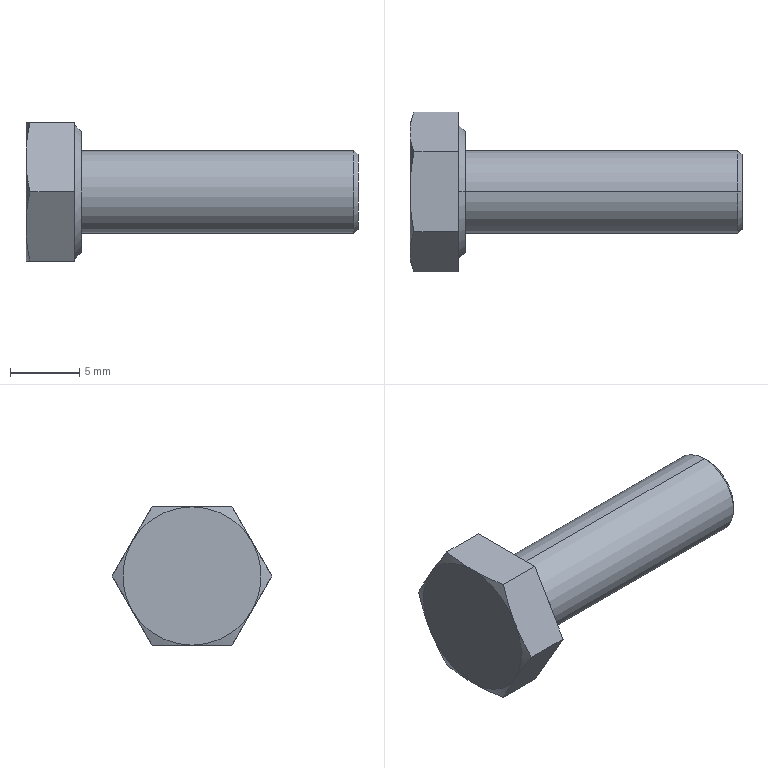Part | STEP file | hex head bolts-full thread grade c gb_GB_FASTENER_BOLT_HHBFTC M6X20-S | 1 solid | 22 faces | box 24 x 11.547 x 10 mm | volume 900.64 mm3 | cone 10 | plane 10 | cylinder 2 | commonest cylinder face diameters 6 x2
STEP:
#1=CARTESIAN_POINT('',(23.7,0.,3.));
#2=VERTEX_POINT('',#1);
#3=CARTESIAN_POINT('',(23.7,0.,-3.));
#4=VERTEX_POINT('',#3);
#5=CARTESIAN_POINT('',(23.7,0.,0.));
#6=DIRECTION('',(-1.,0.,0.));
#7=DIRECTION('',(0.,0.,1.));
#8=AXIS2_PLACEMENT_3D('',#5,#6,#7);
#9=CIRCLE('',#8,3.);
#10=EDGE_CURVE('',#2,#4,#9,.T.);
#11=ORIENTED_EDGE('',*,*,#10,.T.);
#12=CARTESIAN_POINT('',(4.,0.,-3.));
#13=VERTEX_POINT('',#12);
#14=CARTESIAN_POINT('',(24.,0.,-3.));
#15=DIRECTION('',(-1.,0.,0.));
#16=VECTOR('',#15,1000.);
#17=LINE('',#14,#16);
#18=EDGE_CURVE('',#4,#13,#17,.T.);
#19=ORIENTED_EDGE('',*,*,#18,.T.);
#20=CARTESIAN_POINT('',(4.,0.,3.));
#21=VERTEX_POINT('',#20);
#22=CARTESIAN_POINT('',(4.,0.,0.));
#23=DIRECTION('',(1.,0.,0.));
#24=DIRECTION('',(0.,0.,1.));
#25=AXIS2_PLACEMENT_3D('',#22,#23,#24);
#26=CIRCLE('',#25,3.);
#27=EDGE_CURVE('',#13,#21,#26,.T.);
#28=ORIENTED_EDGE('',*,*,#27,.T.);
#29=CARTESIAN_POINT('',(24.,0.,3.));
#30=DIRECTION('',(-1.,0.,0.));
#31=VECTOR('',#30,1000.);
#32=LINE('',#29,#31);
#33=EDGE_CURVE('',#2,#21,#32,.T.);
#34=ORIENTED_EDGE('',*,*,#33,.F.);
#35=EDGE_LOOP('',(#11,#19,#28,#34));
#36=FACE_OUTER_BOUND('',#35,.T.);
#37=CARTESIAN_POINT('',(24.,0.,0.));
#38=DIRECTION('',(-1.,0.,0.));
#39=DIRECTION('',(0.,0.,1.));
#40=AXIS2_PLACEMENT_3D('',#37,#38,#39);
#41=CYLINDRICAL_SURFACE('',#40,3.);
#42=ADVANCED_FACE('',(#36),#41,.T.);
#43=CARTESIAN_POINT('',(24.,0.,2.7));
#44=VERTEX_POINT('',#43);
#45=CARTESIAN_POINT('',(24.,0.,-2.7));
#46=VERTEX_POINT('',#45);
#47=CARTESIAN_POINT('',(24.,0.,0.));
#48=DIRECTION('',(-1.,0.,0.));
#49=DIRECTION('',(0.,0.,1.));
#50=AXIS2_PLACEMENT_3D('',#47,#48,#49);
#51=CIRCLE('',#50,2.7);
#52=EDGE_CURVE('',#44,#46,#51,.T.);
#53=ORIENTED_EDGE('',*,*,#52,.T.);
#54=CARTESIAN_POINT('',(23.7,0.,-3.));
#55=DIRECTION('',(-0.7071,0.,-0.7071));
#56=VECTOR('',#55,1000.);
#57=LINE('',#54,#56);
#58=EDGE_CURVE('',#46,#4,#57,.T.);
#59=ORIENTED_EDGE('',*,*,#58,.T.);
#60=ORIENTED_EDGE('',*,*,#10,.F.);
#61=CARTESIAN_POINT('',(23.7,0.,3.));
#62=DIRECTION('',(-0.7071,0.,0.7071));
#63=VECTOR('',#62,1000.);
#64=LINE('',#61,#63);
#65=EDGE_CURVE('',#44,#2,#64,.T.);
#66=ORIENTED_EDGE('',*,*,#65,.F.);
#67=EDGE_LOOP('',(#53,#59,#60,#66));
#68=FACE_OUTER_BOUND('',#67,.T.);
#69=CARTESIAN_POINT('',(23.7,0.,0.));
#70=DIRECTION('',(-1.,0.,0.));
#71=DIRECTION('',(0.,0.,1.));
#72=AXIS2_PLACEMENT_3D('',#69,#70,#71);
#73=CONICAL_SURFACE('',#72,3.,0.7854);
#74=ADVANCED_FACE('',(#68),#73,.T.);
#75=CARTESIAN_POINT('',(4.,0.,4.37));
#76=VERTEX_POINT('',#75);
#77=CARTESIAN_POINT('',(4.,0.,-4.37));
#78=VERTEX_POINT('',#77);
#79=CARTESIAN_POINT('',(4.,0.,0.));
#80=DIRECTION('',(-1.,0.,0.));
#81=DIRECTION('',(0.,0.,1.));
#82=AXIS2_PLACEMENT_3D('',#79,#80,#81);
#83=CIRCLE('',#82,4.37);
#84=EDGE_CURVE('',#76,#78,#83,.T.);
#85=ORIENTED_EDGE('',*,*,#84,.T.);
#86=CARTESIAN_POINT('',(3.5,0.,-4.87));
#87=VERTEX_POINT('',#86);
#88=CARTESIAN_POINT('',(3.5,0.,-4.87));
#89=DIRECTION('',(-0.7071,0.,-0.7071));
#90=VECTOR('',#89,1000.);
#91=LINE('',#88,#90);
#92=EDGE_CURVE('',#78,#87,#91,.T.);
#93=ORIENTED_EDGE('',*,*,#92,.T.);
#94=CARTESIAN_POINT('',(3.5,0.,4.87));
#95=VERTEX_POINT('',#94);
#96=CARTESIAN_POINT('',(3.5,0.,0.));
#97=DIRECTION('',(1.,0.,0.));
#98=DIRECTION('',(0.,0.,1.));
#99=AXIS2_PLACEMENT_3D('',#96,#97,#98);
#100=CIRCLE('',#99,4.87);
#101=EDGE_CURVE('',#87,#95,#100,.T.);
#102=ORIENTED_EDGE('',*,*,#101,.T.);
#103=CARTESIAN_POINT('',(3.5,0.,4.87));
#104=DIRECTION('',(-0.7071,0.,0.7071));
#105=VECTOR('',#104,1000.);
#106=LINE('',#103,#105);
#107=EDGE_CURVE('',#76,#95,#106,.T.);
#108=ORIENTED_EDGE('',*,*,#107,.F.);
#109=EDGE_LOOP('',(#85,#93,#102,#108));
#110=FACE_OUTER_BOUND('',#109,.T.);
#111=CARTESIAN_POINT('',(3.5,0.,0.));
#112=DIRECTION('',(-1.,0.,0.));
#113=DIRECTION('',(0.,0.,1.));
#114=AXIS2_PLACEMENT_3D('',#111,#112,#113);
#115=CONICAL_SURFACE('',#114,4.87,0.7854);
#116=ADVANCED_FACE('',(#110),#115,.T.);
#117=ORIENTED_EDGE('',*,*,#18,.F.);
#118=CARTESIAN_POINT('',(23.7,0.,0.));
#119=DIRECTION('',(-1.,0.,0.));
#120=DIRECTION('',(0.,0.,1.));
#121=AXIS2_PLACEMENT_3D('',#118,#119,#120);
#122=CIRCLE('',#121,3.);
#123=EDGE_CURVE('',#4,#2,#122,.T.);
#124=ORIENTED_EDGE('',*,*,#123,.T.);
#125=ORIENTED_EDGE('',*,*,#33,.T.);
#126=CARTESIAN_POINT('',(4.,0.,0.));
#127=DIRECTION('',(1.,0.,0.));
#128=DIRECTION('',(0.,0.,1.));
#129=AXIS2_PLACEMENT_3D('',#126,#127,#128);
#130=CIRCLE('',#129,3.);
#131=EDGE_CURVE('',#21,#13,#130,.T.);
#132=ORIENTED_EDGE('',*,*,#131,.T.);
#133=EDGE_LOOP('',(#117,#124,#125,#132));
#134=FACE_OUTER_BOUND('',#133,.T.);
#135=CARTESIAN_POINT('',(24.,0.,0.));
#136=DIRECTION('',(-1.,0.,0.));
#137=DIRECTION('',(0.,0.,1.));
#138=AXIS2_PLACEMENT_3D('',#135,#136,#137);
#139=CYLINDRICAL_SURFACE('',#138,3.);
#140=ADVANCED_FACE('',(#134),#139,.T.);
#141=ORIENTED_EDGE('',*,*,#131,.F.);
#142=ORIENTED_EDGE('',*,*,#27,.F.);
#143=EDGE_LOOP('',(#141,#142));
#144=FACE_BOUND('',#143,.T.);
#145=ORIENTED_EDGE('',*,*,#84,.F.);
#146=CARTESIAN_POINT('',(4.,0.,0.));
#147=DIRECTION('',(-1.,0.,0.));
#148=DIRECTION('',(0.,0.,1.));
#149=AXIS2_PLACEMENT_3D('',#146,#147,#148);
#150=CIRCLE('',#149,4.37);
#151=EDGE_CURVE('',#78,#76,#150,.T.);
#152=ORIENTED_EDGE('',*,*,#151,.F.);
#153=EDGE_LOOP('',(#145,#152));
#154=FACE_OUTER_BOUND('',#153,.T.);
#155=CARTESIAN_POINT('',(4.,0.,10.));
#156=DIRECTION('',(-1.,0.,0.));
#157=DIRECTION('',(0.,0.,1.));
#158=AXIS2_PLACEMENT_3D('',#155,#156,#157);
#159=PLANE('',#158);
#160=ADVANCED_FACE('',(#144,#154),#159,.F.);
#161=ORIENTED_EDGE('',*,*,#58,.F.);
#162=CARTESIAN_POINT('',(24.,0.,0.));
#163=DIRECTION('',(-1.,0.,0.));
#164=DIRECTION('',(0.,0.,1.));
#165=AXIS2_PLACEMENT_3D('',#162,#163,#164);
#166=CIRCLE('',#165,2.7);
#167=EDGE_CURVE('',#46,#44,#166,.T.);
#168=ORIENTED_EDGE('',*,*,#167,.T.);
#169=ORIENTED_EDGE('',*,*,#65,.T.);
#170=ORIENTED_EDGE('',*,*,#123,.F.);
#171=EDGE_LOOP('',(#161,#168,#169,#170));
#172=FACE_OUTER_BOUND('',#171,.T.);
#173=CARTESIAN_POINT('',(23.7,0.,0.));
#174=DIRECTION('',(-1.,0.,0.));
#175=DIRECTION('',(0.,0.,1.));
#176=AXIS2_PLACEMENT_3D('',#173,#174,#175);
#177=CONICAL_SURFACE('',#176,3.,0.7854);
#178=ADVANCED_FACE('',(#172),#177,.T.);
#179=ORIENTED_EDGE('',*,*,#92,.F.);
#180=ORIENTED_EDGE('',*,*,#151,.T.);
#181=ORIENTED_EDGE('',*,*,#107,.T.);
#182=CARTESIAN_POINT('',(3.5,0.,0.));
#183=DIRECTION('',(1.,0.,0.));
#184=DIRECTION('',(0.,0.,1.));
#185=AXIS2_PLACEMENT_3D('',#182,#183,#184);
#186=CIRCLE('',#185,4.87);
#187=EDGE_CURVE('',#95,#87,#186,.T.);
#188=ORIENTED_EDGE('',*,*,#187,.T.);
#189=EDGE_LOOP('',(#179,#180,#181,#188));
#190=FACE_OUTER_BOUND('',#189,.T.);
#191=CARTESIAN_POINT('',(3.5,0.,0.));
#192=DIRECTION('',(-1.,0.,0.));
#193=DIRECTION('',(0.,0.,1.));
#194=AXIS2_PLACEMENT_3D('',#191,#192,#193);
#195=CONICAL_SURFACE('',#194,4.87,0.7854);
#196=ADVANCED_FACE('',(#190),#195,.T.);
#197=ORIENTED_EDGE('',*,*,#52,.F.);
#198=ORIENTED_EDGE('',*,*,#167,.F.);
#199=EDGE_LOOP('',(#197,#198));
#200=FACE_OUTER_BOUND('',#199,.T.);
#201=CARTESIAN_POINT('',(24.,0.,0.));
#202=DIRECTION('',(1.,0.,0.));
#203=DIRECTION('',(0.,0.,-1.));
#204=AXIS2_PLACEMENT_3D('',#201,#202,#203);
#205=PLANE('',#204);
#206=ADVANCED_FACE('',(#200),#205,.T.);
#207=CARTESIAN_POINT('',(3.5,5.774,0.));
#208=VERTEX_POINT('',#207);
#209=CARTESIAN_POINT('',(3.5,2.887,5.));
#210=VERTEX_POINT('',#209);
#211=CARTESIAN_POINT('',(3.5,5.774,0.));
#212=DIRECTION('',(0.,-0.5,0.866));
#213=VECTOR('',#212,1000.);
#214=LINE('',#211,#213);
#215=EDGE_CURVE('',#208,#210,#214,.T.);
#216=ORIENTED_EDGE('',*,*,#215,.T.);
#217=CARTESIAN_POINT('',(3.5,-2.887,5.));
#218=VERTEX_POINT('',#217);
#219=CARTESIAN_POINT('',(3.5,4.87,5.));
#220=DIRECTION('',(0.,-1.,0.));
#221=VECTOR('',#220,1000.);
#222=LINE('',#219,#221);
#223=EDGE_CURVE('',#210,#218,#222,.T.);
#224=ORIENTED_EDGE('',*,*,#223,.T.);
#225=CARTESIAN_POINT('',(3.5,-5.774,0.));
#226=VERTEX_POINT('',#225);
#227=CARTESIAN_POINT('',(3.5,-2.887,5.));
#228=DIRECTION('',(0.,-0.5,-0.866));
#229=VECTOR('',#228,1000.);
#230=LINE('',#227,#229);
#231=EDGE_CURVE('',#218,#226,#230,.T.);
#232=ORIENTED_EDGE('',*,*,#231,.T.);
#233=CARTESIAN_POINT('',(3.5,-2.887,-5.));
#234=VERTEX_POINT('',#233);
#235=CARTESIAN_POINT('',(3.5,-5.774,0.));
#236=DIRECTION('',(0.,0.5,-0.866));
#237=VECTOR('',#236,1000.);
#238=LINE('',#235,#237);
#239=EDGE_CURVE('',#226,#234,#238,.T.);
#240=ORIENTED_EDGE('',*,*,#239,.T.);
#241=CARTESIAN_POINT('',(3.5,2.887,-5.));
#242=VERTEX_POINT('',#241);
#243=CARTESIAN_POINT('',(3.5,4.87,-5.));
#244=DIRECTION('',(0.,1.,0.));
#245=VECTOR('',#244,1000.);
#246=LINE('',#243,#245);
#247=EDGE_CURVE('',#234,#242,#246,.T.);
#248=ORIENTED_EDGE('',*,*,#247,.T.);
#249=CARTESIAN_POINT('',(3.5,2.887,-5.));
#250=DIRECTION('',(0.,0.5,0.866));
#251=VECTOR('',#250,1000.);
#252=LINE('',#249,#251);
#253=EDGE_CURVE('',#242,#208,#252,.T.);
#254=ORIENTED_EDGE('',*,*,#253,.T.);
#255=EDGE_LOOP('',(#216,#224,#232,#240,#248,#254));
#256=FACE_OUTER_BOUND('',#255,.T.);
#257=ORIENTED_EDGE('',*,*,#187,.F.);
#258=ORIENTED_EDGE('',*,*,#101,.F.);
#259=EDGE_LOOP('',(#257,#258));
#260=FACE_BOUND('',#259,.T.);
#261=CARTESIAN_POINT('',(3.5,4.87,0.));
#262=DIRECTION('',(1.,0.,0.));
#263=DIRECTION('',(0.,0.,-1.));
#264=AXIS2_PLACEMENT_3D('',#261,#262,#263);
#265=PLANE('',#264);
#266=ADVANCED_FACE('',(#256,#260),#265,.T.);
#267=CARTESIAN_POINT('',(0.2815,-2.887,5.));
#268=VERTEX_POINT('',#267);
#269=CARTESIAN_POINT('',(4.,-2.887,5.));
#270=DIRECTION('',(-1.,0.,0.));
#271=VECTOR('',#270,1000.);
#272=LINE('',#269,#271);
#273=EDGE_CURVE('',#218,#268,#272,.T.);
#274=ORIENTED_EDGE('',*,*,#273,.F.);
#275=ORIENTED_EDGE('',*,*,#223,.F.);
#276=CARTESIAN_POINT('',(0.2815,2.887,5.));
#277=VERTEX_POINT('',#276);
#278=CARTESIAN_POINT('',(4.,2.887,5.));
#279=DIRECTION('',(1.,0.,0.));
#280=VECTOR('',#279,1000.);
#281=LINE('',#278,#280);
#282=EDGE_CURVE('',#277,#210,#281,.T.);
#283=ORIENTED_EDGE('',*,*,#282,.F.);
#284=CARTESIAN_POINT('',(0.,0.,5.));
#285=VERTEX_POINT('',#284);
#286=CARTESIAN_POINT('',(0.,0.,5.));
#287=CARTESIAN_POINT('',(0.,0.9714,5.));
#288=CARTESIAN_POINT('',(0.1078,1.932,5.));
#289=CARTESIAN_POINT('',(0.2815,2.887,5.));
#290=B_SPLINE_CURVE_WITH_KNOTS('',3,(#286,#287,#288,#289),.UNSPECIFIED.,.F.,.F.,(4,4),(0.,0.0029),.UNSPECIFIED.);
#291=EDGE_CURVE('',#285,#277,#290,.T.);
#292=ORIENTED_EDGE('',*,*,#291,.F.);
#293=CARTESIAN_POINT('',(0.2815,-2.887,5.));
#294=CARTESIAN_POINT('',(0.1078,-1.932,5.));
#295=CARTESIAN_POINT('',(0.,-0.9714,5.));
#296=CARTESIAN_POINT('',(0.,0.,5.));
#297=B_SPLINE_CURVE_WITH_KNOTS('',3,(#293,#294,#295,#296),.UNSPECIFIED.,.F.,.F.,(4,4),(0.,0.0029),.UNSPECIFIED.);
#298=EDGE_CURVE('',#268,#285,#297,.T.);
#299=ORIENTED_EDGE('',*,*,#298,.F.);
#300=EDGE_LOOP('',(#274,#275,#283,#292,#299));
#301=FACE_OUTER_BOUND('',#300,.T.);
#302=CARTESIAN_POINT('',(4.,2.887,5.));
#303=DIRECTION('',(0.,0.,-1.));
#304=DIRECTION('',(0.,1.,0.));
#305=AXIS2_PLACEMENT_3D('',#302,#303,#304);
#306=PLANE('',#305);
#307=ADVANCED_FACE('',(#301),#306,.F.);
#308=ORIENTED_EDGE('',*,*,#282,.T.);
#309=ORIENTED_EDGE('',*,*,#215,.F.);
#310=CARTESIAN_POINT('',(0.2815,5.774,0.));
#311=VERTEX_POINT('',#310);
#312=CARTESIAN_POINT('',(4.,5.774,0.));
#313=DIRECTION('',(1.,0.,0.));
#314=VECTOR('',#313,1000.);
#315=LINE('',#312,#314);
#316=EDGE_CURVE('',#311,#208,#315,.T.);
#317=ORIENTED_EDGE('',*,*,#316,.F.);
#318=CARTESIAN_POINT('',(0.,4.33,2.5));
#319=VERTEX_POINT('',#318);
#320=CARTESIAN_POINT('',(0.,4.33,2.5));
#321=CARTESIAN_POINT('',(0.,4.816,1.659));
#322=CARTESIAN_POINT('',(0.1078,5.296,0.8266));
#323=CARTESIAN_POINT('',(0.2815,5.774,0.));
#324=B_SPLINE_CURVE_WITH_KNOTS('',3,(#320,#321,#322,#323),.UNSPECIFIED.,.F.,.F.,(4,4),(0.,0.0029),.UNSPECIFIED.);
#325=EDGE_CURVE('',#319,#311,#324,.T.);
#326=ORIENTED_EDGE('',*,*,#325,.F.);
#327=CARTESIAN_POINT('',(0.2815,2.887,5.));
#328=CARTESIAN_POINT('',(0.1078,3.364,4.173));
#329=CARTESIAN_POINT('',(0.,3.844,3.341));
#330=CARTESIAN_POINT('',(0.,4.33,2.5));
#331=B_SPLINE_CURVE_WITH_KNOTS('',3,(#327,#328,#329,#330),.UNSPECIFIED.,.F.,.F.,(4,4),(0.,0.0029),.UNSPECIFIED.);
#332=EDGE_CURVE('',#277,#319,#331,.T.);
#333=ORIENTED_EDGE('',*,*,#332,.F.);
#334=EDGE_LOOP('',(#308,#309,#317,#326,#333));
#335=FACE_OUTER_BOUND('',#334,.T.);
#336=CARTESIAN_POINT('',(4.,5.774,0.));
#337=DIRECTION('',(0.,-0.866,-0.5));
#338=DIRECTION('',(0.,0.5,-0.866));
#339=AXIS2_PLACEMENT_3D('',#336,#337,#338);
#340=PLANE('',#339);
#341=ADVANCED_FACE('',(#335),#340,.F.);
#342=ORIENTED_EDGE('',*,*,#316,.T.);
#343=ORIENTED_EDGE('',*,*,#253,.F.);
#344=CARTESIAN_POINT('',(0.2815,2.887,-5.));
#345=VERTEX_POINT('',#344);
#346=CARTESIAN_POINT('',(4.,2.887,-5.));
#347=DIRECTION('',(1.,0.,0.));
#348=VECTOR('',#347,1000.);
#349=LINE('',#346,#348);
#350=EDGE_CURVE('',#345,#242,#349,.T.);
#351=ORIENTED_EDGE('',*,*,#350,.F.);
#352=CARTESIAN_POINT('',(0.,4.33,-2.5));
#353=VERTEX_POINT('',#352);
#354=CARTESIAN_POINT('',(0.,4.33,-2.5));
#355=CARTESIAN_POINT('',(0.,3.844,-3.341));
#356=CARTESIAN_POINT('',(0.1078,3.364,-4.173));
#357=CARTESIAN_POINT('',(0.2815,2.887,-5.));
#358=B_SPLINE_CURVE_WITH_KNOTS('',3,(#354,#355,#356,#357),.UNSPECIFIED.,.F.,.F.,(4,4),(0.,0.0029),.UNSPECIFIED.);
#359=EDGE_CURVE('',#353,#345,#358,.T.);
#360=ORIENTED_EDGE('',*,*,#359,.F.);
#361=CARTESIAN_POINT('',(0.2815,5.774,0.));
#362=CARTESIAN_POINT('',(0.1078,5.296,-0.8266));
#363=CARTESIAN_POINT('',(0.,4.816,-1.659));
#364=CARTESIAN_POINT('',(0.,4.33,-2.5));
#365=B_SPLINE_CURVE_WITH_KNOTS('',3,(#361,#362,#363,#364),.UNSPECIFIED.,.F.,.F.,(4,4),(0.,0.0029),.UNSPECIFIED.);
#366=EDGE_CURVE('',#311,#353,#365,.T.);
#367=ORIENTED_EDGE('',*,*,#366,.F.);
#368=EDGE_LOOP('',(#342,#343,#351,#360,#367));
#369=FACE_OUTER_BOUND('',#368,.T.);
#370=CARTESIAN_POINT('',(4.,2.887,-5.));
#371=DIRECTION('',(0.,-0.866,0.5));
#372=DIRECTION('',(0.,-0.5,-0.866));
#373=AXIS2_PLACEMENT_3D('',#370,#371,#372);
#374=PLANE('',#373);
#375=ADVANCED_FACE('',(#369),#374,.F.);
#376=ORIENTED_EDGE('',*,*,#350,.T.);
#377=ORIENTED_EDGE('',*,*,#247,.F.);
#378=CARTESIAN_POINT('',(0.2815,-2.887,-5.));
#379=VERTEX_POINT('',#378);
#380=CARTESIAN_POINT('',(4.,-2.887,-5.));
#381=DIRECTION('',(1.,0.,0.));
#382=VECTOR('',#381,1000.);
#383=LINE('',#380,#382);
#384=EDGE_CURVE('',#379,#234,#383,.T.);
#385=ORIENTED_EDGE('',*,*,#384,.F.);
#386=CARTESIAN_POINT('',(0.,0.,-5.));
#387=VERTEX_POINT('',#386);
#388=CARTESIAN_POINT('',(0.,0.,-5.));
#389=CARTESIAN_POINT('',(0.,-0.9714,-5.));
#390=CARTESIAN_POINT('',(0.1078,-1.932,-5.));
#391=CARTESIAN_POINT('',(0.2815,-2.887,-5.));
#392=B_SPLINE_CURVE_WITH_KNOTS('',3,(#388,#389,#390,#391),.UNSPECIFIED.,.F.,.F.,(4,4),(0.,0.0029),.UNSPECIFIED.);
#393=EDGE_CURVE('',#387,#379,#392,.T.);
#394=ORIENTED_EDGE('',*,*,#393,.F.);
#395=CARTESIAN_POINT('',(0.2815,2.887,-5.));
#396=CARTESIAN_POINT('',(0.1078,1.932,-5.));
#397=CARTESIAN_POINT('',(0.,0.9714,-5.));
#398=CARTESIAN_POINT('',(0.,0.,-5.));
#399=B_SPLINE_CURVE_WITH_KNOTS('',3,(#395,#396,#397,#398),.UNSPECIFIED.,.F.,.F.,(4,4),(0.,0.0029),.UNSPECIFIED.);
#400=EDGE_CURVE('',#345,#387,#399,.T.);
#401=ORIENTED_EDGE('',*,*,#400,.F.);
#402=EDGE_LOOP('',(#376,#377,#385,#394,#401));
#403=FACE_OUTER_BOUND('',#402,.T.);
#404=CARTESIAN_POINT('',(4.,-2.887,-5.));
#405=DIRECTION('',(0.,0.,1.));
#406=DIRECTION('',(1.,0.,0.));
#407=AXIS2_PLACEMENT_3D('',#404,#405,#406);
#408=PLANE('',#407);
#409=ADVANCED_FACE('',(#403),#408,.F.);
#410=ORIENTED_EDGE('',*,*,#384,.T.);
#411=ORIENTED_EDGE('',*,*,#239,.F.);
#412=CARTESIAN_POINT('',(0.2815,-5.774,0.));
#413=VERTEX_POINT('',#412);
#414=CARTESIAN_POINT('',(4.,-5.774,0.));
#415=DIRECTION('',(1.,0.,0.));
#416=VECTOR('',#415,1000.);
#417=LINE('',#414,#416);
#418=EDGE_CURVE('',#413,#226,#417,.T.);
#419=ORIENTED_EDGE('',*,*,#418,.F.);
#420=CARTESIAN_POINT('',(0.,-4.33,-2.5));
#421=VERTEX_POINT('',#420);
#422=CARTESIAN_POINT('',(0.,-4.33,-2.5));
#423=CARTESIAN_POINT('',(0.,-4.816,-1.659));
#424=CARTESIAN_POINT('',(0.1078,-5.296,-0.8266));
#425=CARTESIAN_POINT('',(0.2815,-5.774,0.));
#426=B_SPLINE_CURVE_WITH_KNOTS('',3,(#422,#423,#424,#425),.UNSPECIFIED.,.F.,.F.,(4,4),(0.,0.0029),.UNSPECIFIED.);
#427=EDGE_CURVE('',#421,#413,#426,.T.);
#428=ORIENTED_EDGE('',*,*,#427,.F.);
#429=CARTESIAN_POINT('',(0.2815,-2.887,-5.));
#430=CARTESIAN_POINT('',(0.1078,-3.364,-4.173));
#431=CARTESIAN_POINT('',(0.,-3.844,-3.341));
#432=CARTESIAN_POINT('',(0.,-4.33,-2.5));
#433=B_SPLINE_CURVE_WITH_KNOTS('',3,(#429,#430,#431,#432),.UNSPECIFIED.,.F.,.F.,(4,4),(0.,0.0029),.UNSPECIFIED.);
#434=EDGE_CURVE('',#379,#421,#433,.T.);
#435=ORIENTED_EDGE('',*,*,#434,.F.);
#436=EDGE_LOOP('',(#410,#411,#419,#428,#435));
#437=FACE_OUTER_BOUND('',#436,.T.);
#438=CARTESIAN_POINT('',(4.,-5.774,0.));
#439=DIRECTION('',(0.,0.866,0.5));
#440=DIRECTION('',(0.,-0.5,0.866));
#441=AXIS2_PLACEMENT_3D('',#438,#439,#440);
#442=PLANE('',#441);
#443=ADVANCED_FACE('',(#437),#442,.F.);
#444=ORIENTED_EDGE('',*,*,#418,.T.);
#445=ORIENTED_EDGE('',*,*,#231,.F.);
#446=ORIENTED_EDGE('',*,*,#273,.T.);
#447=CARTESIAN_POINT('',(0.,-4.33,2.5));
#448=VERTEX_POINT('',#447);
#449=CARTESIAN_POINT('',(0.,-4.33,2.5));
#450=CARTESIAN_POINT('',(0.,-3.844,3.341));
#451=CARTESIAN_POINT('',(0.1078,-3.364,4.173));
#452=CARTESIAN_POINT('',(0.2815,-2.887,5.));
#453=B_SPLINE_CURVE_WITH_KNOTS('',3,(#449,#450,#451,#452),.UNSPECIFIED.,.F.,.F.,(4,4),(0.,0.0029),.UNSPECIFIED.);
#454=EDGE_CURVE('',#448,#268,#453,.T.);
#455=ORIENTED_EDGE('',*,*,#454,.F.);
#456=CARTESIAN_POINT('',(0.2815,-5.774,0.));
#457=CARTESIAN_POINT('',(0.1078,-5.296,0.8266));
#458=CARTESIAN_POINT('',(0.,-4.816,1.659));
#459=CARTESIAN_POINT('',(0.,-4.33,2.5));
#460=B_SPLINE_CURVE_WITH_KNOTS('',3,(#456,#457,#458,#459),.UNSPECIFIED.,.F.,.F.,(4,4),(0.,0.0029),.UNSPECIFIED.);
#461=EDGE_CURVE('',#413,#448,#460,.T.);
#462=ORIENTED_EDGE('',*,*,#461,.F.);
#463=EDGE_LOOP('',(#444,#445,#446,#455,#462));
#464=FACE_OUTER_BOUND('',#463,.T.);
#465=CARTESIAN_POINT('',(4.,-2.887,5.));
#466=DIRECTION('',(0.,0.866,-0.5));
#467=DIRECTION('',(0.,0.5,0.866));
#468=AXIS2_PLACEMENT_3D('',#465,#466,#467);
#469=PLANE('',#468);
#470=ADVANCED_FACE('',(#464),#469,.F.);
#471=ORIENTED_EDGE('',*,*,#298,.T.);
#472=CARTESIAN_POINT('',(0.,0.,0.));
#473=DIRECTION('',(1.,0.,0.));
#474=DIRECTION('',(0.,0.,-1.));
#475=AXIS2_PLACEMENT_3D('',#472,#473,#474);
#476=CIRCLE('',#475,5.);
#477=EDGE_CURVE('',#285,#448,#476,.T.);
#478=ORIENTED_EDGE('',*,*,#477,.T.);
#479=ORIENTED_EDGE('',*,*,#454,.T.);
#480=EDGE_LOOP('',(#471,#478,#479));
#481=FACE_OUTER_BOUND('',#480,.T.);
#482=CARTESIAN_POINT('',(0.2832,0.,0.));
#483=DIRECTION('',(1.,0.,0.));
#484=DIRECTION('',(0.,0.,-1.));
#485=AXIS2_PLACEMENT_3D('',#482,#483,#484);
#486=CONICAL_SURFACE('',#485,5.778,1.222);
#487=ADVANCED_FACE('',(#481),#486,.T.);
#488=CARTESIAN_POINT('',(0.,0.,0.));
#489=DIRECTION('',(1.,0.,0.));
#490=DIRECTION('',(0.,0.,-1.));
#491=AXIS2_PLACEMENT_3D('',#488,#489,#490);
#492=CIRCLE('',#491,5.);
#493=EDGE_CURVE('',#319,#285,#492,.T.);
#494=ORIENTED_EDGE('',*,*,#493,.T.);
#495=ORIENTED_EDGE('',*,*,#291,.T.);
#496=ORIENTED_EDGE('',*,*,#332,.T.);
#497=EDGE_LOOP('',(#494,#495,#496));
#498=FACE_OUTER_BOUND('',#497,.T.);
#499=CARTESIAN_POINT('',(0.2832,0.,0.));
#500=DIRECTION('',(1.,0.,0.));
#501=DIRECTION('',(0.,0.,-1.));
#502=AXIS2_PLACEMENT_3D('',#499,#500,#501);
#503=CONICAL_SURFACE('',#502,5.778,1.222);
#504=ADVANCED_FACE('',(#498),#503,.T.);
#505=CARTESIAN_POINT('',(0.,0.,0.));
#506=DIRECTION('',(1.,0.,0.));
#507=DIRECTION('',(0.,0.,-1.));
#508=AXIS2_PLACEMENT_3D('',#505,#506,#507);
#509=CIRCLE('',#508,5.);
#510=EDGE_CURVE('',#353,#319,#509,.T.);
#511=ORIENTED_EDGE('',*,*,#510,.T.);
#512=ORIENTED_EDGE('',*,*,#325,.T.);
#513=ORIENTED_EDGE('',*,*,#366,.T.);
#514=EDGE_LOOP('',(#511,#512,#513));
#515=FACE_OUTER_BOUND('',#514,.T.);
#516=CARTESIAN_POINT('',(0.2832,0.,0.));
#517=DIRECTION('',(1.,0.,0.));
#518=DIRECTION('',(0.,0.,-1.));
#519=AXIS2_PLACEMENT_3D('',#516,#517,#518);
#520=CONICAL_SURFACE('',#519,5.778,1.222);
#521=ADVANCED_FACE('',(#515),#520,.T.);
#522=CARTESIAN_POINT('',(0.,0.,0.));
#523=DIRECTION('',(1.,0.,0.));
#524=DIRECTION('',(0.,0.,-1.));
#525=AXIS2_PLACEMENT_3D('',#522,#523,#524);
#526=CIRCLE('',#525,5.);
#527=EDGE_CURVE('',#387,#353,#526,.T.);
#528=ORIENTED_EDGE('',*,*,#527,.T.);
#529=ORIENTED_EDGE('',*,*,#359,.T.);
#530=ORIENTED_EDGE('',*,*,#400,.T.);
#531=EDGE_LOOP('',(#528,#529,#530));
#532=FACE_OUTER_BOUND('',#531,.T.);
#533=CARTESIAN_POINT('',(0.2832,0.,0.));
#534=DIRECTION('',(1.,0.,0.));
#535=DIRECTION('',(0.,0.,-1.));
#536=AXIS2_PLACEMENT_3D('',#533,#534,#535);
#537=CONICAL_SURFACE('',#536,5.778,1.222);
#538=ADVANCED_FACE('',(#532),#537,.T.);
#539=ORIENTED_EDGE('',*,*,#434,.T.);
#540=CARTESIAN_POINT('',(0.,0.,0.));
#541=DIRECTION('',(1.,0.,0.));
#542=DIRECTION('',(0.,0.,-1.));
#543=AXIS2_PLACEMENT_3D('',#540,#541,#542);
#544=CIRCLE('',#543,5.);
#545=EDGE_CURVE('',#421,#387,#544,.T.);
#546=ORIENTED_EDGE('',*,*,#545,.T.);
#547=ORIENTED_EDGE('',*,*,#393,.T.);
#548=EDGE_LOOP('',(#539,#546,#547));
#549=FACE_OUTER_BOUND('',#548,.T.);
#550=CARTESIAN_POINT('',(0.2832,0.,0.));
#551=DIRECTION('',(1.,0.,0.));
#552=DIRECTION('',(0.,0.,-1.));
#553=AXIS2_PLACEMENT_3D('',#550,#551,#552);
#554=CONICAL_SURFACE('',#553,5.778,1.222);
#555=ADVANCED_FACE('',(#549),#554,.T.);
#556=ORIENTED_EDGE('',*,*,#461,.T.);
#557=CARTESIAN_POINT('',(0.,0.,0.));
#558=DIRECTION('',(1.,0.,0.));
#559=DIRECTION('',(0.,0.,-1.));
#560=AXIS2_PLACEMENT_3D('',#557,#558,#559);
#561=CIRCLE('',#560,5.);
#562=EDGE_CURVE('',#448,#421,#561,.T.);
#563=ORIENTED_EDGE('',*,*,#562,.T.);
#564=ORIENTED_EDGE('',*,*,#427,.T.);
#565=EDGE_LOOP('',(#556,#563,#564));
#566=FACE_OUTER_BOUND('',#565,.T.);
#567=CARTESIAN_POINT('',(0.2832,0.,0.));
#568=DIRECTION('',(1.,0.,0.));
#569=DIRECTION('',(0.,0.,-1.));
#570=AXIS2_PLACEMENT_3D('',#567,#568,#569);
#571=CONICAL_SURFACE('',#570,5.778,1.222);
#572=ADVANCED_FACE('',(#566),#571,.T.);
#573=ORIENTED_EDGE('',*,*,#545,.F.);
#574=ORIENTED_EDGE('',*,*,#562,.F.);
#575=ORIENTED_EDGE('',*,*,#477,.F.);
#576=ORIENTED_EDGE('',*,*,#493,.F.);
#577=ORIENTED_EDGE('',*,*,#510,.F.);
#578=ORIENTED_EDGE('',*,*,#527,.F.);
#579=EDGE_LOOP('',(#573,#574,#575,#576,#577,#578));
#580=FACE_OUTER_BOUND('',#579,.T.);
#581=CARTESIAN_POINT('',(0.,0.,10.));
#582=DIRECTION('',(-1.,0.,0.));
#583=DIRECTION('',(0.,0.,1.));
#584=AXIS2_PLACEMENT_3D('',#581,#582,#583);
#585=PLANE('',#584);
#586=ADVANCED_FACE('',(#580),#585,.T.);
#587=CLOSED_SHELL('',(#42,#74,#116,#140,#160,#178,#196,#206,#266,#307,#341,#375,#409,#443,#470,#487,#504,#521,#538,#555,#572,#586));
#588=MANIFOLD_SOLID_BREP('',#587);
#589=CARTESIAN_POINT('',(0.,0.,0.));
#590=DIRECTION('',(0.,0.,1.));
#591=DIRECTION('',(1.,0.,0.));
#592=AXIS2_PLACEMENT_3D('',#589,#590,#591);
#593=(LENGTH_UNIT()NAMED_UNIT(*)SI_UNIT(.MILLI.,.METRE.));
#594=UNCERTAINTY_MEASURE_WITH_UNIT(LENGTH_MEASURE(0.00001),#593,'','');
#595=(NAMED_UNIT(*)PLANE_ANGLE_UNIT()SI_UNIT($,.RADIAN.));
#596=(NAMED_UNIT(*)SI_UNIT($,.STERADIAN.)SOLID_ANGLE_UNIT());
#597=(GEOMETRIC_REPRESENTATION_CONTEXT(3)GLOBAL_UNCERTAINTY_ASSIGNED_CONTEXT((#594))GLOBAL_UNIT_ASSIGNED_CONTEXT((#593,#595,#596))REPRESENTATION_CONTEXT('',''));
#598=ADVANCED_BREP_SHAPE_REPRESENTATION('',(#588,#592),#597);